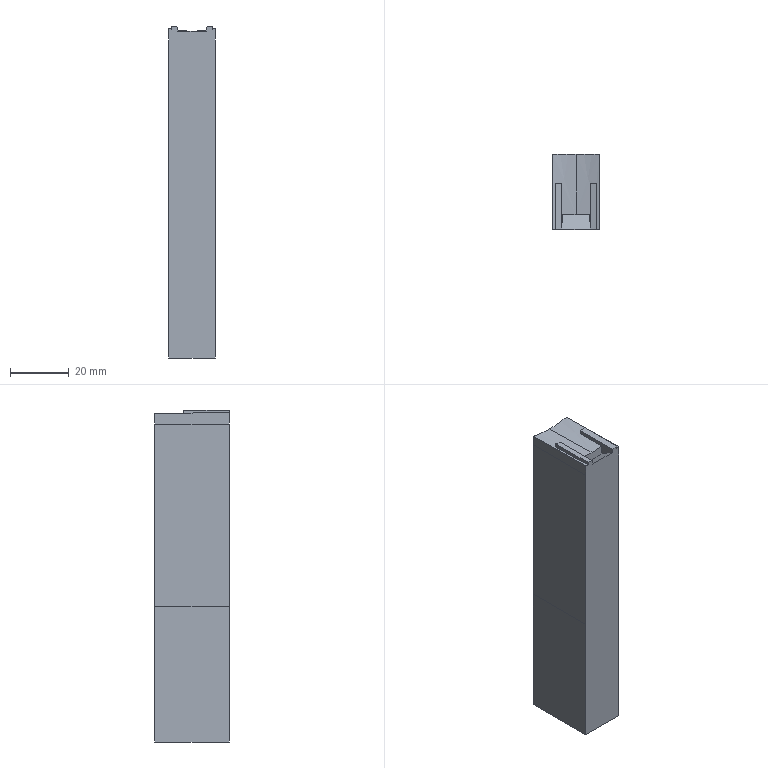Part | STEP file | Core - Tower - Drawer insert 2 - 1 cav | 1 solid | 21 faces | box 16.003 x 25.438 x 113.201 mm | volume 45404 mm3 | plane 17 | cone 2 | cylinder 2 | commonest cylinder face diameters 67.284 x2